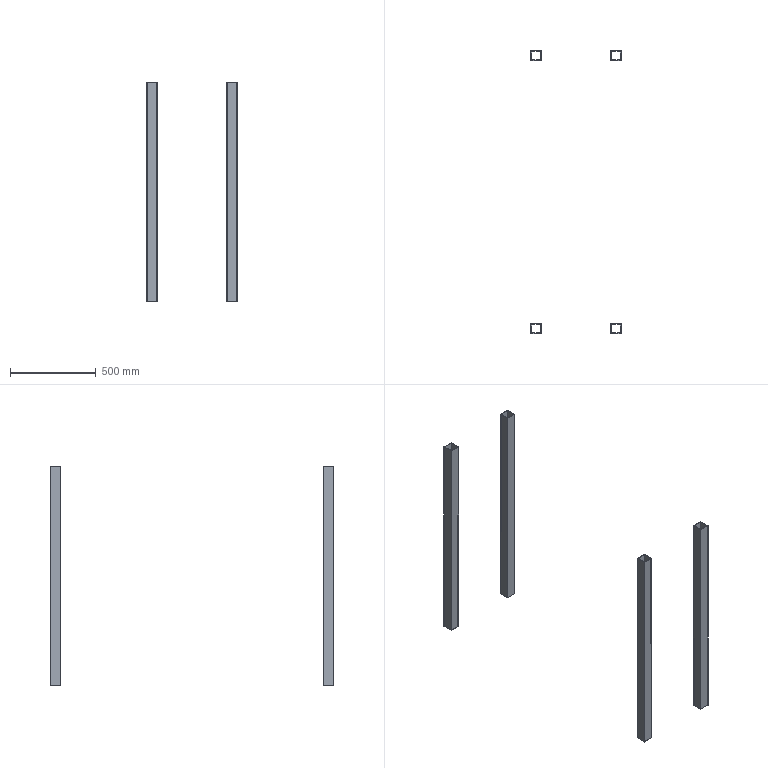Part | STEP file | ASND-0110-E63-HLTP01标准Lower机架-02 | 4 solids | 64 faces | box 525 x 1650 x 1280 mm | volume 4586578 mm3 | plane 40 | cylinder 24 | commonest cylinder face diameters 5 x24